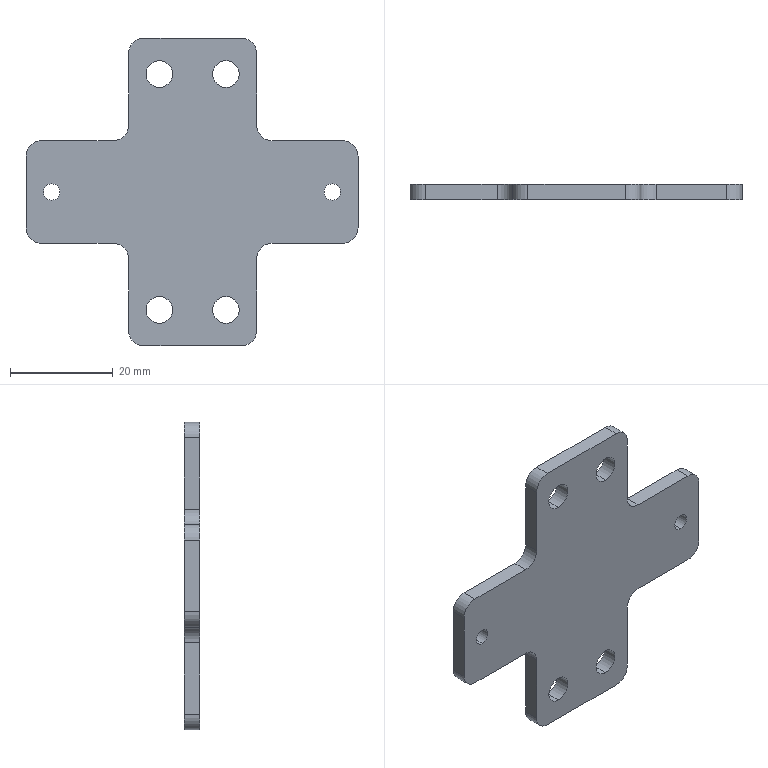Part | SolidWorks | features BaseBody 1 | 1 solid | 38 faces | box 64.75 x 3 x 60 mm | volume 6559 mm3 | cylinder 24 | plane 14 | commonest cylinder face diameters 6 x12 5.2 x8 3.2 x4
STEP:
#1=CARTESIAN_POINT('',(39.75,0.,-31.6));
#2=VERTEX_POINT('',#1);
#3=CARTESIAN_POINT('',(39.75,0.,-28.4));
#4=VERTEX_POINT('',#3);
#5=CARTESIAN_POINT('',(39.75,0.,-30.));
#6=DIRECTION('',(0.,1.,0.));
#7=DIRECTION('',(0.,0.,1.));
#8=AXIS2_PLACEMENT_3D('',#5,#6,#7);
#9=CIRCLE('',#8,1.6);
#10=EDGE_CURVE('',#2,#4,#9,.T.);
#11=ORIENTED_EDGE('',*,*,#10,.F.);
#12=CARTESIAN_POINT('',(39.75,3.,-31.6));
#13=VERTEX_POINT('',#12);
#14=CARTESIAN_POINT('',(39.75,-28.284,-31.6));
#15=DIRECTION('',(0.,1.,0.));
#16=VECTOR('',#15,1000.);
#17=LINE('',#14,#16);
#18=EDGE_CURVE('',#2,#13,#17,.T.);
#19=ORIENTED_EDGE('',*,*,#18,.T.);
#20=CARTESIAN_POINT('',(39.75,3.,-28.4));
#21=VERTEX_POINT('',#20);
#22=CARTESIAN_POINT('',(39.75,3.,-30.));
#23=DIRECTION('',(0.,-1.,0.));
#24=DIRECTION('',(0.,0.,1.));
#25=AXIS2_PLACEMENT_3D('',#22,#23,#24);
#26=CIRCLE('',#25,1.6);
#27=EDGE_CURVE('',#21,#13,#26,.T.);
#28=ORIENTED_EDGE('',*,*,#27,.F.);
#29=CARTESIAN_POINT('',(39.75,-28.284,-28.4));
#30=DIRECTION('',(0.,1.,0.));
#31=VECTOR('',#30,1000.);
#32=LINE('',#29,#31);
#33=EDGE_CURVE('',#4,#21,#32,.T.);
#34=ORIENTED_EDGE('',*,*,#33,.F.);
#35=EDGE_LOOP('',(#11,#19,#28,#34));
#36=FACE_OUTER_BOUND('',#35,.T.);
#37=CARTESIAN_POINT('',(39.75,-28.284,-30.));
#38=DIRECTION('',(0.,1.,0.));
#39=DIRECTION('',(0.,0.,1.));
#40=AXIS2_PLACEMENT_3D('',#37,#38,#39);
#41=CYLINDRICAL_SURFACE('',#40,1.6);
#42=ADVANCED_FACE('',(#36),#41,.F.);
#43=CARTESIAN_POINT('',(-15.,0.,-31.6));
#44=VERTEX_POINT('',#43);
#45=CARTESIAN_POINT('',(-15.,0.,-28.4));
#46=VERTEX_POINT('',#45);
#47=CARTESIAN_POINT('',(-15.,0.,-30.));
#48=DIRECTION('',(0.,1.,0.));
#49=DIRECTION('',(0.,0.,1.));
#50=AXIS2_PLACEMENT_3D('',#47,#48,#49);
#51=CIRCLE('',#50,1.6);
#52=EDGE_CURVE('',#44,#46,#51,.T.);
#53=ORIENTED_EDGE('',*,*,#52,.F.);
#54=CARTESIAN_POINT('',(-15.,3.,-31.6));
#55=VERTEX_POINT('',#54);
#56=CARTESIAN_POINT('',(-15.,-28.284,-31.6));
#57=DIRECTION('',(0.,1.,0.));
#58=VECTOR('',#57,1000.);
#59=LINE('',#56,#58);
#60=EDGE_CURVE('',#44,#55,#59,.T.);
#61=ORIENTED_EDGE('',*,*,#60,.T.);
#62=CARTESIAN_POINT('',(-15.,3.,-28.4));
#63=VERTEX_POINT('',#62);
#64=CARTESIAN_POINT('',(-15.,3.,-30.));
#65=DIRECTION('',(0.,-1.,0.));
#66=DIRECTION('',(0.,0.,1.));
#67=AXIS2_PLACEMENT_3D('',#64,#65,#66);
#68=CIRCLE('',#67,1.6);
#69=EDGE_CURVE('',#63,#55,#68,.T.);
#70=ORIENTED_EDGE('',*,*,#69,.F.);
#71=CARTESIAN_POINT('',(-15.,-28.284,-28.4));
#72=DIRECTION('',(0.,1.,0.));
#73=VECTOR('',#72,1000.);
#74=LINE('',#71,#73);
#75=EDGE_CURVE('',#46,#63,#74,.T.);
#76=ORIENTED_EDGE('',*,*,#75,.F.);
#77=EDGE_LOOP('',(#53,#61,#70,#76));
#78=FACE_OUTER_BOUND('',#77,.T.);
#79=CARTESIAN_POINT('',(-15.,-28.284,-30.));
#80=DIRECTION('',(0.,1.,0.));
#81=DIRECTION('',(0.,0.,1.));
#82=AXIS2_PLACEMENT_3D('',#79,#80,#81);
#83=CYLINDRICAL_SURFACE('',#82,1.6);
#84=ADVANCED_FACE('',(#78),#83,.F.);
#85=CARTESIAN_POINT('',(19.,3.,-50.4));
#86=VERTEX_POINT('',#85);
#87=CARTESIAN_POINT('',(19.,3.,-55.6));
#88=VERTEX_POINT('',#87);
#89=CARTESIAN_POINT('',(19.,3.,-53.));
#90=DIRECTION('',(0.,-1.,0.));
#91=DIRECTION('',(0.,0.,-1.));
#92=AXIS2_PLACEMENT_3D('',#89,#90,#91);
#93=CIRCLE('',#92,2.6);
#94=EDGE_CURVE('',#86,#88,#93,.T.);
#95=ORIENTED_EDGE('',*,*,#94,.F.);
#96=CARTESIAN_POINT('',(19.,0.,-50.4));
#97=VERTEX_POINT('',#96);
#98=CARTESIAN_POINT('',(19.,3.,-50.4));
#99=DIRECTION('',(0.,-1.,0.));
#100=VECTOR('',#99,1000.);
#101=LINE('',#98,#100);
#102=EDGE_CURVE('',#86,#97,#101,.T.);
#103=ORIENTED_EDGE('',*,*,#102,.T.);
#104=CARTESIAN_POINT('',(19.,0.,-55.6));
#105=VERTEX_POINT('',#104);
#106=CARTESIAN_POINT('',(19.,0.,-53.));
#107=DIRECTION('',(0.,1.,0.));
#108=DIRECTION('',(0.,0.,-1.));
#109=AXIS2_PLACEMENT_3D('',#106,#107,#108);
#110=CIRCLE('',#109,2.6);
#111=EDGE_CURVE('',#105,#97,#110,.T.);
#112=ORIENTED_EDGE('',*,*,#111,.F.);
#113=CARTESIAN_POINT('',(19.,3.,-55.6));
#114=DIRECTION('',(0.,-1.,0.));
#115=VECTOR('',#114,1000.);
#116=LINE('',#113,#115);
#117=EDGE_CURVE('',#88,#105,#116,.T.);
#118=ORIENTED_EDGE('',*,*,#117,.F.);
#119=EDGE_LOOP('',(#95,#103,#112,#118));
#120=FACE_OUTER_BOUND('',#119,.T.);
#121=CARTESIAN_POINT('',(19.,3.,-53.));
#122=DIRECTION('',(0.,-1.,0.));
#123=DIRECTION('',(0.,0.,-1.));
#124=AXIS2_PLACEMENT_3D('',#121,#122,#123);
#125=CYLINDRICAL_SURFACE('',#124,2.6);
#126=ADVANCED_FACE('',(#120),#125,.F.);
#127=CARTESIAN_POINT('',(19.,3.,-4.4));
#128=VERTEX_POINT('',#127);
#129=CARTESIAN_POINT('',(19.,3.,-9.6));
#130=VERTEX_POINT('',#129);
#131=CARTESIAN_POINT('',(19.,3.,-7.));
#132=DIRECTION('',(0.,-1.,0.));
#133=DIRECTION('',(0.,0.,-1.));
#134=AXIS2_PLACEMENT_3D('',#131,#132,#133);
#135=CIRCLE('',#134,2.6);
#136=EDGE_CURVE('',#128,#130,#135,.T.);
#137=ORIENTED_EDGE('',*,*,#136,.F.);
#138=CARTESIAN_POINT('',(19.,0.,-4.4));
#139=VERTEX_POINT('',#138);
#140=CARTESIAN_POINT('',(19.,3.,-4.4));
#141=DIRECTION('',(0.,-1.,0.));
#142=VECTOR('',#141,1000.);
#143=LINE('',#140,#142);
#144=EDGE_CURVE('',#128,#139,#143,.T.);
#145=ORIENTED_EDGE('',*,*,#144,.T.);
#146=CARTESIAN_POINT('',(19.,0.,-9.6));
#147=VERTEX_POINT('',#146);
#148=CARTESIAN_POINT('',(19.,0.,-7.));
#149=DIRECTION('',(0.,1.,0.));
#150=DIRECTION('',(0.,0.,-1.));
#151=AXIS2_PLACEMENT_3D('',#148,#149,#150);
#152=CIRCLE('',#151,2.6);
#153=EDGE_CURVE('',#147,#139,#152,.T.);
#154=ORIENTED_EDGE('',*,*,#153,.F.);
#155=CARTESIAN_POINT('',(19.,3.,-9.6));
#156=DIRECTION('',(0.,-1.,0.));
#157=VECTOR('',#156,1000.);
#158=LINE('',#155,#157);
#159=EDGE_CURVE('',#130,#147,#158,.T.);
#160=ORIENTED_EDGE('',*,*,#159,.F.);
#161=EDGE_LOOP('',(#137,#145,#154,#160));
#162=FACE_OUTER_BOUND('',#161,.T.);
#163=CARTESIAN_POINT('',(19.,3.,-7.));
#164=DIRECTION('',(0.,-1.,0.));
#165=DIRECTION('',(0.,0.,-1.));
#166=AXIS2_PLACEMENT_3D('',#163,#164,#165);
#167=CYLINDRICAL_SURFACE('',#166,2.6);
#168=ADVANCED_FACE('',(#162),#167,.F.);
#169=CARTESIAN_POINT('',(6.,3.,-4.4));
#170=VERTEX_POINT('',#169);
#171=CARTESIAN_POINT('',(6.,3.,-9.6));
#172=VERTEX_POINT('',#171);
#173=CARTESIAN_POINT('',(6.,3.,-7.));
#174=DIRECTION('',(0.,-1.,0.));
#175=DIRECTION('',(0.,0.,-1.));
#176=AXIS2_PLACEMENT_3D('',#173,#174,#175);
#177=CIRCLE('',#176,2.6);
#178=EDGE_CURVE('',#170,#172,#177,.T.);
#179=ORIENTED_EDGE('',*,*,#178,.F.);
#180=CARTESIAN_POINT('',(6.,0.,-4.4));
#181=VERTEX_POINT('',#180);
#182=CARTESIAN_POINT('',(6.,3.,-4.4));
#183=DIRECTION('',(0.,-1.,0.));
#184=VECTOR('',#183,1000.);
#185=LINE('',#182,#184);
#186=EDGE_CURVE('',#170,#181,#185,.T.);
#187=ORIENTED_EDGE('',*,*,#186,.T.);
#188=CARTESIAN_POINT('',(6.,0.,-9.6));
#189=VERTEX_POINT('',#188);
#190=CARTESIAN_POINT('',(6.,0.,-7.));
#191=DIRECTION('',(0.,1.,0.));
#192=DIRECTION('',(0.,0.,-1.));
#193=AXIS2_PLACEMENT_3D('',#190,#191,#192);
#194=CIRCLE('',#193,2.6);
#195=EDGE_CURVE('',#189,#181,#194,.T.);
#196=ORIENTED_EDGE('',*,*,#195,.F.);
#197=CARTESIAN_POINT('',(6.,3.,-9.6));
#198=DIRECTION('',(0.,-1.,0.));
#199=VECTOR('',#198,1000.);
#200=LINE('',#197,#199);
#201=EDGE_CURVE('',#172,#189,#200,.T.);
#202=ORIENTED_EDGE('',*,*,#201,.F.);
#203=EDGE_LOOP('',(#179,#187,#196,#202));
#204=FACE_OUTER_BOUND('',#203,.T.);
#205=CARTESIAN_POINT('',(6.,3.,-7.));
#206=DIRECTION('',(0.,-1.,0.));
#207=DIRECTION('',(0.,0.,-1.));
#208=AXIS2_PLACEMENT_3D('',#205,#206,#207);
#209=CYLINDRICAL_SURFACE('',#208,2.6);
#210=ADVANCED_FACE('',(#204),#209,.F.);
#211=CARTESIAN_POINT('',(6.,3.,-50.4));
#212=VERTEX_POINT('',#211);
#213=CARTESIAN_POINT('',(6.,3.,-55.6));
#214=VERTEX_POINT('',#213);
#215=CARTESIAN_POINT('',(6.,3.,-53.));
#216=DIRECTION('',(0.,-1.,0.));
#217=DIRECTION('',(0.,0.,-1.));
#218=AXIS2_PLACEMENT_3D('',#215,#216,#217);
#219=CIRCLE('',#218,2.6);
#220=EDGE_CURVE('',#212,#214,#219,.T.);
#221=ORIENTED_EDGE('',*,*,#220,.F.);
#222=CARTESIAN_POINT('',(6.,0.,-50.4));
#223=VERTEX_POINT('',#222);
#224=CARTESIAN_POINT('',(6.,3.,-50.4));
#225=DIRECTION('',(0.,-1.,0.));
#226=VECTOR('',#225,1000.);
#227=LINE('',#224,#226);
#228=EDGE_CURVE('',#212,#223,#227,.T.);
#229=ORIENTED_EDGE('',*,*,#228,.T.);
#230=CARTESIAN_POINT('',(6.,0.,-55.6));
#231=VERTEX_POINT('',#230);
#232=CARTESIAN_POINT('',(6.,0.,-53.));
#233=DIRECTION('',(0.,1.,0.));
#234=DIRECTION('',(0.,0.,-1.));
#235=AXIS2_PLACEMENT_3D('',#232,#233,#234);
#236=CIRCLE('',#235,2.6);
#237=EDGE_CURVE('',#231,#223,#236,.T.);
#238=ORIENTED_EDGE('',*,*,#237,.F.);
#239=CARTESIAN_POINT('',(6.,3.,-55.6));
#240=DIRECTION('',(0.,-1.,0.));
#241=VECTOR('',#240,1000.);
#242=LINE('',#239,#241);
#243=EDGE_CURVE('',#214,#231,#242,.T.);
#244=ORIENTED_EDGE('',*,*,#243,.F.);
#245=EDGE_LOOP('',(#221,#229,#238,#244));
#246=FACE_OUTER_BOUND('',#245,.T.);
#247=CARTESIAN_POINT('',(6.,3.,-53.));
#248=DIRECTION('',(0.,-1.,0.));
#249=DIRECTION('',(0.,0.,-1.));
#250=AXIS2_PLACEMENT_3D('',#247,#248,#249);
#251=CYLINDRICAL_SURFACE('',#250,2.6);
#252=ADVANCED_FACE('',(#246),#251,.F.);
#253=CARTESIAN_POINT('',(39.75,0.,-30.));
#254=DIRECTION('',(0.,1.,0.));
#255=DIRECTION('',(0.,0.,1.));
#256=AXIS2_PLACEMENT_3D('',#253,#254,#255);
#257=CIRCLE('',#256,1.6);
#258=EDGE_CURVE('',#4,#2,#257,.T.);
#259=ORIENTED_EDGE('',*,*,#258,.T.);
#260=ORIENTED_EDGE('',*,*,#10,.T.);
#261=EDGE_LOOP('',(#259,#260));
#262=FACE_BOUND('',#261,.T.);
#263=CARTESIAN_POINT('',(-15.,0.,-30.));
#264=DIRECTION('',(0.,1.,0.));
#265=DIRECTION('',(0.,0.,1.));
#266=AXIS2_PLACEMENT_3D('',#263,#264,#265);
#267=CIRCLE('',#266,1.6);
#268=EDGE_CURVE('',#46,#44,#267,.T.);
#269=ORIENTED_EDGE('',*,*,#268,.T.);
#270=ORIENTED_EDGE('',*,*,#52,.T.);
#271=EDGE_LOOP('',(#269,#270));
#272=FACE_BOUND('',#271,.T.);
#273=ORIENTED_EDGE('',*,*,#111,.T.);
#274=CARTESIAN_POINT('',(19.,0.,-53.));
#275=DIRECTION('',(0.,1.,0.));
#276=DIRECTION('',(0.,0.,-1.));
#277=AXIS2_PLACEMENT_3D('',#274,#275,#276);
#278=CIRCLE('',#277,2.6);
#279=EDGE_CURVE('',#97,#105,#278,.T.);
#280=ORIENTED_EDGE('',*,*,#279,.T.);
#281=EDGE_LOOP('',(#273,#280));
#282=FACE_BOUND('',#281,.T.);
#283=ORIENTED_EDGE('',*,*,#153,.T.);
#284=CARTESIAN_POINT('',(19.,0.,-7.));
#285=DIRECTION('',(0.,1.,0.));
#286=DIRECTION('',(0.,0.,-1.));
#287=AXIS2_PLACEMENT_3D('',#284,#285,#286);
#288=CIRCLE('',#287,2.6);
#289=EDGE_CURVE('',#139,#147,#288,.T.);
#290=ORIENTED_EDGE('',*,*,#289,.T.);
#291=EDGE_LOOP('',(#283,#290));
#292=FACE_BOUND('',#291,.T.);
#293=CARTESIAN_POINT('',(28.,0.,-40.));
#294=VERTEX_POINT('',#293);
#295=CARTESIAN_POINT('',(41.75,0.,-40.));
#296=VERTEX_POINT('',#295);
#297=CARTESIAN_POINT('',(0.,0.,-40.));
#298=DIRECTION('',(1.,0.,0.));
#299=VECTOR('',#298,1000.);
#300=LINE('',#297,#299);
#301=EDGE_CURVE('',#294,#296,#300,.T.);
#302=ORIENTED_EDGE('',*,*,#301,.T.);
#303=CARTESIAN_POINT('',(44.75,0.,-37.));
#304=VERTEX_POINT('',#303);
#305=CARTESIAN_POINT('',(41.75,0.,-37.));
#306=DIRECTION('',(0.,-1.,0.));
#307=DIRECTION('',(0.,0.,1.));
#308=AXIS2_PLACEMENT_3D('',#305,#306,#307);
#309=CIRCLE('',#308,3.);
#310=EDGE_CURVE('',#296,#304,#309,.T.);
#311=ORIENTED_EDGE('',*,*,#310,.T.);
#312=CARTESIAN_POINT('',(44.75,0.,-23.));
#313=VERTEX_POINT('',#312);
#314=CARTESIAN_POINT('',(44.75,0.,0.));
#315=DIRECTION('',(0.,0.,1.));
#316=VECTOR('',#315,1000.);
#317=LINE('',#314,#316);
#318=EDGE_CURVE('',#304,#313,#317,.T.);
#319=ORIENTED_EDGE('',*,*,#318,.T.);
#320=CARTESIAN_POINT('',(41.75,0.,-20.));
#321=VERTEX_POINT('',#320);
#322=CARTESIAN_POINT('',(41.75,0.,-23.));
#323=DIRECTION('',(0.,-1.,0.));
#324=DIRECTION('',(0.,0.,1.));
#325=AXIS2_PLACEMENT_3D('',#322,#323,#324);
#326=CIRCLE('',#325,3.);
#327=EDGE_CURVE('',#313,#321,#326,.T.);
#328=ORIENTED_EDGE('',*,*,#327,.T.);
#329=CARTESIAN_POINT('',(28.,0.,-20.));
#330=VERTEX_POINT('',#329);
#331=CARTESIAN_POINT('',(0.,0.,-20.));
#332=DIRECTION('',(-1.,0.,0.));
#333=VECTOR('',#332,1000.);
#334=LINE('',#331,#333);
#335=EDGE_CURVE('',#321,#330,#334,.T.);
#336=ORIENTED_EDGE('',*,*,#335,.T.);
#337=CARTESIAN_POINT('',(25.,0.,-17.));
#338=VERTEX_POINT('',#337);
#339=CARTESIAN_POINT('',(28.,0.,-17.));
#340=DIRECTION('',(0.,1.,0.));
#341=DIRECTION('',(0.,0.,1.));
#342=AXIS2_PLACEMENT_3D('',#339,#340,#341);
#343=CIRCLE('',#342,3.);
#344=EDGE_CURVE('',#330,#338,#343,.T.);
#345=ORIENTED_EDGE('',*,*,#344,.T.);
#346=CARTESIAN_POINT('',(25.,0.,-3.));
#347=VERTEX_POINT('',#346);
#348=CARTESIAN_POINT('',(25.,0.,0.));
#349=DIRECTION('',(0.,0.,1.));
#350=VECTOR('',#349,1000.);
#351=LINE('',#348,#350);
#352=EDGE_CURVE('',#338,#347,#351,.T.);
#353=ORIENTED_EDGE('',*,*,#352,.T.);
#354=CARTESIAN_POINT('',(22.,0.,0.));
#355=VERTEX_POINT('',#354);
#356=CARTESIAN_POINT('',(22.,0.,-3.));
#357=DIRECTION('',(0.,-1.,0.));
#358=DIRECTION('',(0.,0.,-1.));
#359=AXIS2_PLACEMENT_3D('',#356,#357,#358);
#360=CIRCLE('',#359,3.);
#361=EDGE_CURVE('',#347,#355,#360,.T.);
#362=ORIENTED_EDGE('',*,*,#361,.T.);
#363=CARTESIAN_POINT('',(3.,0.,0.));
#364=VERTEX_POINT('',#363);
#365=CARTESIAN_POINT('',(0.,0.,0.));
#366=DIRECTION('',(-1.,0.,0.));
#367=VECTOR('',#366,1000.);
#368=LINE('',#365,#367);
#369=EDGE_CURVE('',#355,#364,#368,.T.);
#370=ORIENTED_EDGE('',*,*,#369,.T.);
#371=CARTESIAN_POINT('',(0.,0.,-3.));
#372=VERTEX_POINT('',#371);
#373=CARTESIAN_POINT('',(3.,0.,-3.));
#374=DIRECTION('',(0.,-1.,0.));
#375=DIRECTION('',(0.,0.,-1.));
#376=AXIS2_PLACEMENT_3D('',#373,#374,#375);
#377=CIRCLE('',#376,3.);
#378=EDGE_CURVE('',#364,#372,#377,.T.);
#379=ORIENTED_EDGE('',*,*,#378,.T.);
#380=CARTESIAN_POINT('',(0.,0.,-17.));
#381=VERTEX_POINT('',#380);
#382=CARTESIAN_POINT('',(0.,0.,0.));
#383=DIRECTION('',(0.,0.,-1.));
#384=VECTOR('',#383,1000.);
#385=LINE('',#382,#384);
#386=EDGE_CURVE('',#372,#381,#385,.T.);
#387=ORIENTED_EDGE('',*,*,#386,.T.);
#388=CARTESIAN_POINT('',(-3.,0.,-20.));
#389=VERTEX_POINT('',#388);
#390=CARTESIAN_POINT('',(-3.,0.,-17.));
#391=DIRECTION('',(0.,1.,0.));
#392=DIRECTION('',(0.,0.,1.));
#393=AXIS2_PLACEMENT_3D('',#390,#391,#392);
#394=CIRCLE('',#393,3.);
#395=EDGE_CURVE('',#381,#389,#394,.T.);
#396=ORIENTED_EDGE('',*,*,#395,.T.);
#397=CARTESIAN_POINT('',(-17.,0.,-20.));
#398=VERTEX_POINT('',#397);
#399=CARTESIAN_POINT('',(0.,0.,-20.));
#400=DIRECTION('',(-1.,0.,0.));
#401=VECTOR('',#400,1000.);
#402=LINE('',#399,#401);
#403=EDGE_CURVE('',#389,#398,#402,.T.);
#404=ORIENTED_EDGE('',*,*,#403,.T.);
#405=CARTESIAN_POINT('',(-20.,0.,-23.));
#406=VERTEX_POINT('',#405);
#407=CARTESIAN_POINT('',(-17.,0.,-23.));
#408=DIRECTION('',(0.,-1.,0.));
#409=DIRECTION('',(0.,0.,1.));
#410=AXIS2_PLACEMENT_3D('',#407,#408,#409);
#411=CIRCLE('',#410,3.);
#412=EDGE_CURVE('',#398,#406,#411,.T.);
#413=ORIENTED_EDGE('',*,*,#412,.T.);
#414=CARTESIAN_POINT('',(-20.,0.,-37.));
#415=VERTEX_POINT('',#414);
#416=CARTESIAN_POINT('',(-20.,0.,0.));
#417=DIRECTION('',(0.,0.,-1.));
#418=VECTOR('',#417,1000.);
#419=LINE('',#416,#418);
#420=EDGE_CURVE('',#406,#415,#419,.T.);
#421=ORIENTED_EDGE('',*,*,#420,.T.);
#422=CARTESIAN_POINT('',(-17.,0.,-40.));
#423=VERTEX_POINT('',#422);
#424=CARTESIAN_POINT('',(-17.,0.,-37.));
#425=DIRECTION('',(0.,-1.,0.));
#426=DIRECTION('',(0.,0.,1.));
#427=AXIS2_PLACEMENT_3D('',#424,#425,#426);
#428=CIRCLE('',#427,3.);
#429=EDGE_CURVE('',#415,#423,#428,.T.);
#430=ORIENTED_EDGE('',*,*,#429,.T.);
#431=CARTESIAN_POINT('',(-3.,0.,-40.));
#432=VERTEX_POINT('',#431);
#433=CARTESIAN_POINT('',(0.,0.,-40.));
#434=DIRECTION('',(1.,0.,0.));
#435=VECTOR('',#434,1000.);
#436=LINE('',#433,#435);
#437=EDGE_CURVE('',#423,#432,#436,.T.);
#438=ORIENTED_EDGE('',*,*,#437,.T.);
#439=CARTESIAN_POINT('',(0.,0.,-43.));
#440=VERTEX_POINT('',#439);
#441=CARTESIAN_POINT('',(-3.,0.,-43.));
#442=DIRECTION('',(0.,1.,0.));
#443=DIRECTION('',(0.,0.,1.));
#444=AXIS2_PLACEMENT_3D('',#441,#442,#443);
#445=CIRCLE('',#444,3.);
#446=EDGE_CURVE('',#432,#440,#445,.T.);
#447=ORIENTED_EDGE('',*,*,#446,.T.);
#448=CARTESIAN_POINT('',(0.,0.,-57.));
#449=VERTEX_POINT('',#448);
#450=CARTESIAN_POINT('',(0.,0.,0.));
#451=DIRECTION('',(0.,0.,-1.));
#452=VECTOR('',#451,1000.);
#453=LINE('',#450,#452);
#454=EDGE_CURVE('',#440,#449,#453,.T.);
#455=ORIENTED_EDGE('',*,*,#454,.T.);
#456=CARTESIAN_POINT('',(3.,0.,-60.));
#457=VERTEX_POINT('',#456);
#458=CARTESIAN_POINT('',(3.,0.,-57.));
#459=DIRECTION('',(0.,-1.,0.));
#460=DIRECTION('',(0.,0.,-1.));
#461=AXIS2_PLACEMENT_3D('',#458,#459,#460);
#462=CIRCLE('',#461,3.);
#463=EDGE_CURVE('',#449,#457,#462,.T.);
#464=ORIENTED_EDGE('',*,*,#463,.T.);
#465=CARTESIAN_POINT('',(22.,0.,-60.));
#466=VERTEX_POINT('',#465);
#467=CARTESIAN_POINT('',(0.,0.,-60.));
#468=DIRECTION('',(1.,0.,0.));
#469=VECTOR('',#468,1000.);
#470=LINE('',#467,#469);
#471=EDGE_CURVE('',#457,#466,#470,.T.);
#472=ORIENTED_EDGE('',*,*,#471,.T.);
#473=CARTESIAN_POINT('',(25.,0.,-57.));
#474=VERTEX_POINT('',#473);
#475=CARTESIAN_POINT('',(22.,0.,-57.));
#476=DIRECTION('',(0.,-1.,0.));
#477=DIRECTION('',(0.,0.,-1.));
#478=AXIS2_PLACEMENT_3D('',#475,#476,#477);
#479=CIRCLE('',#478,3.);
#480=EDGE_CURVE('',#466,#474,#479,.T.);
#481=ORIENTED_EDGE('',*,*,#480,.T.);
#482=CARTESIAN_POINT('',(25.,0.,-43.));
#483=VERTEX_POINT('',#482);
#484=CARTESIAN_POINT('',(25.,0.,0.));
#485=DIRECTION('',(0.,0.,1.));
#486=VECTOR('',#485,1000.);
#487=LINE('',#484,#486);
#488=EDGE_CURVE('',#474,#483,#487,.T.);
#489=ORIENTED_EDGE('',*,*,#488,.T.);
#490=CARTESIAN_POINT('',(28.,0.,-43.));
#491=DIRECTION('',(0.,1.,0.));
#492=DIRECTION('',(0.,0.,1.));
#493=AXIS2_PLACEMENT_3D('',#490,#491,#492);
#494=CIRCLE('',#493,3.);
#495=EDGE_CURVE('',#483,#294,#494,.T.);
#496=ORIENTED_EDGE('',*,*,#495,.T.);
#497=EDGE_LOOP('',(#302,#311,#319,#328,#336,#345,#353,#362,#370,#379,#387,#396,#404,#413,#421,#430,#438,#447,#455,#464,#472,#481,#489,#496));
#498=FACE_OUTER_BOUND('',#497,.T.);
#499=ORIENTED_EDGE('',*,*,#195,.T.);
#500=CARTESIAN_POINT('',(6.,0.,-7.));
#501=DIRECTION('',(0.,1.,0.));
#502=DIRECTION('',(0.,0.,-1.));
#503=AXIS2_PLACEMENT_3D('',#500,#501,#502);
#504=CIRCLE('',#503,2.6);
#505=EDGE_CURVE('',#181,#189,#504,.T.);
#506=ORIENTED_EDGE('',*,*,#505,.T.);
#507=EDGE_LOOP('',(#499,#506));
#508=FACE_BOUND('',#507,.T.);
#509=ORIENTED_EDGE('',*,*,#237,.T.);
#510=CARTESIAN_POINT('',(6.,0.,-53.));
#511=DIRECTION('',(0.,1.,0.));
#512=DIRECTION('',(0.,0.,-1.));
#513=AXIS2_PLACEMENT_3D('',#510,#511,#512);
#514=CIRCLE('',#513,2.6);
#515=EDGE_CURVE('',#223,#231,#514,.T.);
#516=ORIENTED_EDGE('',*,*,#515,.T.);
#517=EDGE_LOOP('',(#509,#516));
#518=FACE_BOUND('',#517,.T.);
#519=CARTESIAN_POINT('',(0.,0.,0.));
#520=DIRECTION('',(0.,-1.,0.));
#521=DIRECTION('',(0.,0.,-1.));
#522=AXIS2_PLACEMENT_3D('',#519,#520,#521);
#523=PLANE('',#522);
#524=ADVANCED_FACE('',(#262,#272,#282,#292,#498,#508,#518),#523,.T.);
#525=ORIENTED_EDGE('',*,*,#18,.F.);
#526=ORIENTED_EDGE('',*,*,#258,.F.);
#527=ORIENTED_EDGE('',*,*,#33,.T.);
#528=CARTESIAN_POINT('',(39.75,3.,-30.));
#529=DIRECTION('',(0.,-1.,0.));
#530=DIRECTION('',(0.,0.,1.));
#531=AXIS2_PLACEMENT_3D('',#528,#529,#530);
#532=CIRCLE('',#531,1.6);
#533=EDGE_CURVE('',#13,#21,#532,.T.);
#534=ORIENTED_EDGE('',*,*,#533,.F.);
#535=EDGE_LOOP('',(#525,#526,#527,#534));
#536=FACE_OUTER_BOUND('',#535,.T.);
#537=CARTESIAN_POINT('',(39.75,-28.284,-30.));
#538=DIRECTION('',(0.,1.,0.));
#539=DIRECTION('',(0.,0.,1.));
#540=AXIS2_PLACEMENT_3D('',#537,#538,#539);
#541=CYLINDRICAL_SURFACE('',#540,1.6);
#542=ADVANCED_FACE('',(#536),#541,.F.);
#543=ORIENTED_EDGE('',*,*,#60,.F.);
#544=ORIENTED_EDGE('',*,*,#268,.F.);
#545=ORIENTED_EDGE('',*,*,#75,.T.);
#546=CARTESIAN_POINT('',(-15.,3.,-30.));
#547=DIRECTION('',(0.,-1.,0.));
#548=DIRECTION('',(0.,0.,1.));
#549=AXIS2_PLACEMENT_3D('',#546,#547,#548);
#550=CIRCLE('',#549,1.6);
#551=EDGE_CURVE('',#55,#63,#550,.T.);
#552=ORIENTED_EDGE('',*,*,#551,.F.);
#553=EDGE_LOOP('',(#543,#544,#545,#552));
#554=FACE_OUTER_BOUND('',#553,.T.);
#555=CARTESIAN_POINT('',(-15.,-28.284,-30.));
#556=DIRECTION('',(0.,1.,0.));
#557=DIRECTION('',(0.,0.,1.));
#558=AXIS2_PLACEMENT_3D('',#555,#556,#557);
#559=CYLINDRICAL_SURFACE('',#558,1.6);
#560=ADVANCED_FACE('',(#554),#559,.F.);
#561=ORIENTED_EDGE('',*,*,#102,.F.);
#562=CARTESIAN_POINT('',(19.,3.,-53.));
#563=DIRECTION('',(0.,-1.,0.));
#564=DIRECTION('',(0.,0.,-1.));
#565=AXIS2_PLACEMENT_3D('',#562,#563,#564);
#566=CIRCLE('',#565,2.6);
#567=EDGE_CURVE('',#88,#86,#566,.T.);
#568=ORIENTED_EDGE('',*,*,#567,.F.);
#569=ORIENTED_EDGE('',*,*,#117,.T.);
#570=ORIENTED_EDGE('',*,*,#279,.F.);
#571=EDGE_LOOP('',(#561,#568,#569,#570));
#572=FACE_OUTER_BOUND('',#571,.T.);
#573=CARTESIAN_POINT('',(19.,3.,-53.));
#574=DIRECTION('',(0.,-1.,0.));
#575=DIRECTION('',(0.,0.,-1.));
#576=AXIS2_PLACEMENT_3D('',#573,#574,#575);
#577=CYLINDRICAL_SURFACE('',#576,2.6);
#578=ADVANCED_FACE('',(#572),#577,.F.);
#579=ORIENTED_EDGE('',*,*,#144,.F.);
#580=CARTESIAN_POINT('',(19.,3.,-7.));
#581=DIRECTION('',(0.,-1.,0.));
#582=DIRECTION('',(0.,0.,-1.));
#583=AXIS2_PLACEMENT_3D('',#580,#581,#582);
#584=CIRCLE('',#583,2.6);
#585=EDGE_CURVE('',#130,#128,#584,.T.);
#586=ORIENTED_EDGE('',*,*,#585,.F.);
#587=ORIENTED_EDGE('',*,*,#159,.T.);
#588=ORIENTED_EDGE('',*,*,#289,.F.);
#589=EDGE_LOOP('',(#579,#586,#587,#588));
#590=FACE_OUTER_BOUND('',#589,.T.);
#591=CARTESIAN_POINT('',(19.,3.,-7.));
#592=DIRECTION('',(0.,-1.,0.));
#593=DIRECTION('',(0.,0.,-1.));
#594=AXIS2_PLACEMENT_3D('',#591,#592,#593);
#595=CYLINDRICAL_SURFACE('',#594,2.6);
#596=ADVANCED_FACE('',(#590),#595,.F.);
#597=CARTESIAN_POINT('',(41.75,3.,-40.));
#598=VERTEX_POINT('',#597);
#599=CARTESIAN_POINT('',(44.75,3.,-37.));
#600=VERTEX_POINT('',#599);
#601=CARTESIAN_POINT('',(41.75,3.,-37.));
#602=DIRECTION('',(0.,-1.,0.));
#603=DIRECTION('',(0.,0.,1.));
#604=AXIS2_PLACEMENT_3D('',#601,#602,#603);
#605=CIRCLE('',#604,3.);
#606=EDGE_CURVE('',#598,#600,#605,.T.);
#607=ORIENTED_EDGE('',*,*,#606,.T.);
#608=CARTESIAN_POINT('',(44.75,-28.284,-37.));
#609=DIRECTION('',(0.,-1.,0.));
#610=VECTOR('',#609,1000.);
#611=LINE('',#608,#610);
#612=EDGE_CURVE('',#600,#304,#611,.T.);
#613=ORIENTED_EDGE('',*,*,#612,.T.);
#614=ORIENTED_EDGE('',*,*,#310,.F.);
#615=CARTESIAN_POINT('',(41.75,-28.284,-40.));
#616=DIRECTION('',(0.,1.,0.));
#617=VECTOR('',#616,1000.);
#618=LINE('',#615,#617);
#619=EDGE_CURVE('',#296,#598,#618,.T.);
#620=ORIENTED_EDGE('',*,*,#619,.T.);
#621=EDGE_LOOP('',(#607,#613,#614,#620));
#622=FACE_OUTER_BOUND('',#621,.T.);
#623=CARTESIAN_POINT('',(41.75,-28.284,-37.));
#624=DIRECTION('',(0.,1.,0.));
#625=DIRECTION('',(0.,0.,1.));
#626=AXIS2_PLACEMENT_3D('',#623,#624,#625);
#627=CYLINDRICAL_SURFACE('',#626,3.);
#628=ADVANCED_FACE('',(#622),#627,.T.);
#629=ORIENTED_EDGE('',*,*,#301,.F.);
#630=CARTESIAN_POINT('',(28.,3.,-40.));
#631=VERTEX_POINT('',#630);
#632=CARTESIAN_POINT('',(28.,-28.284,-40.));
#633=DIRECTION('',(0.,1.,0.));
#634=VECTOR('',#633,1000.);
#635=LINE('',#632,#634);
#636=EDGE_CURVE('',#294,#631,#635,.T.);
#637=ORIENTED_EDGE('',*,*,#636,.T.);
#638=CARTESIAN_POINT('',(25.,3.,-40.));
#639=DIRECTION('',(1.,0.,0.));
#640=VECTOR('',#639,1000.);
#641=LINE('',#638,#640);
#642=EDGE_CURVE('',#631,#598,#641,.T.);
#643=ORIENTED_EDGE('',*,*,#642,.T.);
#644=ORIENTED_EDGE('',*,*,#619,.F.);
#645=EDGE_LOOP('',(#629,#637,#643,#644));
#646=FACE_OUTER_BOUND('',#645,.T.);
#647=CARTESIAN_POINT('',(25.,-28.284,-40.));
#648=DIRECTION('',(0.,0.,-1.));
#649=DIRECTION('',(-1.,0.,0.));
#650=AXIS2_PLACEMENT_3D('',#647,#648,#649);
#651=PLANE('',#650);
#652=ADVANCED_FACE('',(#646),#651,.T.);
#653=CARTESIAN_POINT('',(25.,3.,-43.));
#654=VERTEX_POINT('',#653);
#655=CARTESIAN_POINT('',(25.,-28.284,-43.));
#656=DIRECTION('',(0.,-1.,0.));
#657=VECTOR('',#656,1000.);
#658=LINE('',#655,#657);
#659=EDGE_CURVE('',#654,#483,#658,.T.);
#660=ORIENTED_EDGE('',*,*,#659,.F.);
#661=CARTESIAN_POINT('',(28.,3.,-43.));
#662=DIRECTION('',(0.,-1.,0.));
#663=DIRECTION('',(0.,0.,1.));
#664=AXIS2_PLACEMENT_3D('',#661,#662,#663);
#665=CIRCLE('',#664,3.);
#666=EDGE_CURVE('',#631,#654,#665,.T.);
#667=ORIENTED_EDGE('',*,*,#666,.F.);
#668=ORIENTED_EDGE('',*,*,#636,.F.);
#669=ORIENTED_EDGE('',*,*,#495,.F.);
#670=EDGE_LOOP('',(#660,#667,#668,#669));
#671=FACE_OUTER_BOUND('',#670,.T.);
#672=CARTESIAN_POINT('',(28.,-28.284,-43.));
#673=DIRECTION('',(0.,1.,0.));
#674=DIRECTION('',(0.,0.,1.));
#675=AXIS2_PLACEMENT_3D('',#672,#673,#674);
#676=CYLINDRICAL_SURFACE('',#675,3.);
#677=ADVANCED_FACE('',(#671),#676,.F.);
#678=ORIENTED_EDGE('',*,*,#659,.T.);
#679=ORIENTED_EDGE('',*,*,#488,.F.);
#680=CARTESIAN_POINT('',(25.,3.,-57.));
#681=VERTEX_POINT('',#680);
#682=CARTESIAN_POINT('',(25.,3.,-57.));
#683=DIRECTION('',(0.,-1.,0.));
#684=VECTOR('',#683,1000.);
#685=LINE('',#682,#684);
#686=EDGE_CURVE('',#681,#474,#685,.T.);
#687=ORIENTED_EDGE('',*,*,#686,.F.);
#688=CARTESIAN_POINT('',(25.,3.,0.));
#689=DIRECTION('',(0.,0.,-1.));
#690=VECTOR('',#689,1000.);
#691=LINE('',#688,#690);
#692=EDGE_CURVE('',#654,#681,#691,.T.);
#693=ORIENTED_EDGE('',*,*,#692,.F.);
#694=EDGE_LOOP('',(#678,#679,#687,#693));
#695=FACE_OUTER_BOUND('',#694,.T.);
#696=CARTESIAN_POINT('',(25.,3.,0.));
#697=DIRECTION('',(-1.,0.,0.));
#698=DIRECTION('',(0.,0.,1.));
#699=AXIS2_PLACEMENT_3D('',#696,#697,#698);
#700=PLANE('',#699);
#701=ADVANCED_FACE('',(#695),#700,.F.);
#702=ORIENTED_EDGE('',*,*,#480,.F.);
#703=CARTESIAN_POINT('',(22.,3.,-60.));
#704=VERTEX_POINT('',#703);
#705=CARTESIAN_POINT('',(22.,3.,-60.));
#706=DIRECTION('',(0.,1.,0.));
#707=VECTOR('',#706,1000.);
#708=LINE('',#705,#707);
#709=EDGE_CURVE('',#466,#704,#708,.T.);
#710=ORIENTED_EDGE('',*,*,#709,.T.);
#711=CARTESIAN_POINT('',(22.,3.,-57.));
#712=DIRECTION('',(0.,-1.,0.));
#713=DIRECTION('',(0.,0.,-1.));
#714=AXIS2_PLACEMENT_3D('',#711,#712,#713);
#715=CIRCLE('',#714,3.);
#716=EDGE_CURVE('',#704,#681,#715,.T.);
#717=ORIENTED_EDGE('',*,*,#716,.T.);
#718=ORIENTED_EDGE('',*,*,#686,.T.);
#719=EDGE_LOOP('',(#702,#710,#717,#718));
#720=FACE_OUTER_BOUND('',#719,.T.);
#721=CARTESIAN_POINT('',(22.,3.,-57.));
#722=DIRECTION('',(0.,-1.,0.));
#723=DIRECTION('',(0.,0.,-1.));
#724=AXIS2_PLACEMENT_3D('',#721,#722,#723);
#725=CYLINDRICAL_SURFACE('',#724,3.);
#726=ADVANCED_FACE('',(#720),#725,.T.);
#727=ORIENTED_EDGE('',*,*,#709,.F.);
#728=ORIENTED_EDGE('',*,*,#471,.F.);
#729=CARTESIAN_POINT('',(3.,3.,-60.));
#730=VERTEX_POINT('',#729);
#731=CARTESIAN_POINT('',(3.,3.,-60.));
#732=DIRECTION('',(0.,-1.,0.));
#733=VECTOR('',#732,1000.);
#734=LINE('',#731,#733);
#735=EDGE_CURVE('',#730,#457,#734,.T.);
#736=ORIENTED_EDGE('',*,*,#735,.F.);
#737=CARTESIAN_POINT('',(0.,3.,-60.));
#738=DIRECTION('',(-1.,0.,0.));
#739=VECTOR('',#738,1000.);
#740=LINE('',#737,#739);
#741=EDGE_CURVE('',#704,#730,#740,.T.);
#742=ORIENTED_EDGE('',*,*,#741,.F.);
#743=EDGE_LOOP('',(#727,#728,#736,#742));
#744=FACE_OUTER_BOUND('',#743,.T.);
#745=CARTESIAN_POINT('',(0.,3.,-60.));
#746=DIRECTION('',(0.,0.,1.));
#747=DIRECTION('',(1.,0.,0.));
#748=AXIS2_PLACEMENT_3D('',#745,#746,#747);
#749=PLANE('',#748);
#750=ADVANCED_FACE('',(#744),#749,.F.);
#751=ORIENTED_EDGE('',*,*,#463,.F.);
#752=CARTESIAN_POINT('',(0.,3.,-57.));
#753=VERTEX_POINT('',#752);
#754=CARTESIAN_POINT('',(0.,3.,-57.));
#755=DIRECTION('',(0.,1.,0.));
#756=VECTOR('',#755,1000.);
#757=LINE('',#754,#756);
#758=EDGE_CURVE('',#449,#753,#757,.T.);
#759=ORIENTED_EDGE('',*,*,#758,.T.);
#760=CARTESIAN_POINT('',(3.,3.,-57.));
#761=DIRECTION('',(0.,-1.,0.));
#762=DIRECTION('',(0.,0.,-1.));
#763=AXIS2_PLACEMENT_3D('',#760,#761,#762);
#764=CIRCLE('',#763,3.);
#765=EDGE_CURVE('',#753,#730,#764,.T.);
#766=ORIENTED_EDGE('',*,*,#765,.T.);
#767=ORIENTED_EDGE('',*,*,#735,.T.);
#768=EDGE_LOOP('',(#751,#759,#766,#767));
#769=FACE_OUTER_BOUND('',#768,.T.);
#770=CARTESIAN_POINT('',(3.,3.,-57.));
#771=DIRECTION('',(0.,-1.,0.));
#772=DIRECTION('',(0.,0.,-1.));
#773=AXIS2_PLACEMENT_3D('',#770,#771,#772);
#774=CYLINDRICAL_SURFACE('',#773,3.);
#775=ADVANCED_FACE('',(#769),#774,.T.);
#776=ORIENTED_EDGE('',*,*,#758,.F.);
#777=ORIENTED_EDGE('',*,*,#454,.F.);
#778=CARTESIAN_POINT('',(0.,3.,-43.));
#779=VERTEX_POINT('',#778);
#780=CARTESIAN_POINT('',(0.,3.,-43.));
#781=DIRECTION('',(0.,-1.,0.));
#782=VECTOR('',#781,1000.);
#783=LINE('',#780,#782);
#784=EDGE_CURVE('',#779,#440,#783,.T.);
#785=ORIENTED_EDGE('',*,*,#784,.F.);
#786=CARTESIAN_POINT('',(0.,3.,0.));
#787=DIRECTION('',(0.,0.,1.));
#788=VECTOR('',#787,1000.);
#789=LINE('',#786,#788);
#790=EDGE_CURVE('',#753,#779,#789,.T.);
#791=ORIENTED_EDGE('',*,*,#790,.F.);
#792=EDGE_LOOP('',(#776,#777,#785,#791));
#793=FACE_OUTER_BOUND('',#792,.T.);
#794=CARTESIAN_POINT('',(0.,3.,0.));
#795=DIRECTION('',(1.,0.,0.));
#796=DIRECTION('',(0.,0.,-1.));
#797=AXIS2_PLACEMENT_3D('',#794,#795,#796);
#798=PLANE('',#797);
#799=ADVANCED_FACE('',(#793),#798,.F.);
#800=CARTESIAN_POINT('',(-3.,3.,-40.));
#801=VERTEX_POINT('',#800);
#802=CARTESIAN_POINT('',(-3.,3.,-40.));
#803=DIRECTION('',(0.,-1.,0.));
#804=VECTOR('',#803,1000.);
#805=LINE('',#802,#804);
#806=EDGE_CURVE('',#801,#432,#805,.T.);
#807=ORIENTED_EDGE('',*,*,#806,.F.);
#808=CARTESIAN_POINT('',(-3.,3.,-43.));
#809=DIRECTION('',(0.,-1.,0.));
#810=DIRECTION('',(0.,0.,1.));
#811=AXIS2_PLACEMENT_3D('',#808,#809,#810);
#812=CIRCLE('',#811,3.);
#813=EDGE_CURVE('',#779,#801,#812,.T.);
#814=ORIENTED_EDGE('',*,*,#813,.F.);
#815=ORIENTED_EDGE('',*,*,#784,.T.);
#816=ORIENTED_EDGE('',*,*,#446,.F.);
#817=EDGE_LOOP('',(#807,#814,#815,#816));
#818=FACE_OUTER_BOUND('',#817,.T.);
#819=CARTESIAN_POINT('',(-3.,3.,-43.));
#820=DIRECTION('',(0.,1.,0.));
#821=DIRECTION('',(0.,0.,1.));
#822=AXIS2_PLACEMENT_3D('',#819,#820,#821);
#823=CYLINDRICAL_SURFACE('',#822,3.);
#824=ADVANCED_FACE('',(#818),#823,.F.);
#825=ORIENTED_EDGE('',*,*,#437,.F.);
#826=CARTESIAN_POINT('',(-17.,3.,-40.));
#827=VERTEX_POINT('',#826);
#828=CARTESIAN_POINT('',(-17.,-28.284,-40.));
#829=DIRECTION('',(0.,1.,0.));
#830=VECTOR('',#829,1000.);
#831=LINE('',#828,#830);
#832=EDGE_CURVE('',#423,#827,#831,.T.);
#833=ORIENTED_EDGE('',*,*,#832,.T.);
#834=CARTESIAN_POINT('',(0.,3.,-40.));
#835=DIRECTION('',(1.,0.,0.));
#836=VECTOR('',#835,1000.);
#837=LINE('',#834,#836);
#838=EDGE_CURVE('',#827,#801,#837,.T.);
#839=ORIENTED_EDGE('',*,*,#838,.T.);
#840=ORIENTED_EDGE('',*,*,#806,.T.);
#841=EDGE_LOOP('',(#825,#833,#839,#840));
#842=FACE_OUTER_BOUND('',#841,.T.);
#843=CARTESIAN_POINT('',(0.,-28.284,-40.));
#844=DIRECTION('',(0.,0.,-1.));
#845=DIRECTION('',(-1.,0.,0.));
#846=AXIS2_PLACEMENT_3D('',#843,#844,#845);
#847=PLANE('',#846);
#848=ADVANCED_FACE('',(#842),#847,.T.);
#849=CARTESIAN_POINT('',(-20.,3.,-37.));
#850=VERTEX_POINT('',#849);
#851=CARTESIAN_POINT('',(-17.,3.,-37.));
#852=DIRECTION('',(0.,-1.,0.));
#853=DIRECTION('',(0.,0.,1.));
#854=AXIS2_PLACEMENT_3D('',#851,#852,#853);
#855=CIRCLE('',#854,3.);
#856=EDGE_CURVE('',#850,#827,#855,.T.);
#857=ORIENTED_EDGE('',*,*,#856,.T.);
#858=ORIENTED_EDGE('',*,*,#832,.F.);
#859=ORIENTED_EDGE('',*,*,#429,.F.);
#860=CARTESIAN_POINT('',(-20.,-28.284,-37.));
#861=DIRECTION('',(0.,1.,0.));
#862=VECTOR('',#861,1000.);
#863=LINE('',#860,#862);
#864=EDGE_CURVE('',#415,#850,#863,.T.);
#865=ORIENTED_EDGE('',*,*,#864,.T.);
#866=EDGE_LOOP('',(#857,#858,#859,#865));
#867=FACE_OUTER_BOUND('',#866,.T.);
#868=CARTESIAN_POINT('',(-17.,-28.284,-37.));
#869=DIRECTION('',(0.,1.,0.));
#870=DIRECTION('',(0.,0.,1.));
#871=AXIS2_PLACEMENT_3D('',#868,#869,#870);
#872=CYLINDRICAL_SURFACE('',#871,3.);
#873=ADVANCED_FACE('',(#867),#872,.T.);
#874=ORIENTED_EDGE('',*,*,#420,.F.);
#875=CARTESIAN_POINT('',(-20.,3.,-23.));
#876=VERTEX_POINT('',#875);
#877=CARTESIAN_POINT('',(-20.,-28.284,-23.));
#878=DIRECTION('',(0.,1.,0.));
#879=VECTOR('',#878,1000.);
#880=LINE('',#877,#879);
#881=EDGE_CURVE('',#406,#876,#880,.T.);
#882=ORIENTED_EDGE('',*,*,#881,.T.);
#883=CARTESIAN_POINT('',(-20.,3.,-40.));
#884=DIRECTION('',(0.,0.,-1.));
#885=VECTOR('',#884,1000.);
#886=LINE('',#883,#885);
#887=EDGE_CURVE('',#876,#850,#886,.T.);
#888=ORIENTED_EDGE('',*,*,#887,.T.);
#889=ORIENTED_EDGE('',*,*,#864,.F.);
#890=EDGE_LOOP('',(#874,#882,#888,#889));
#891=FACE_OUTER_BOUND('',#890,.T.);
#892=CARTESIAN_POINT('',(-20.,-28.284,-40.));
#893=DIRECTION('',(-1.,0.,0.));
#894=DIRECTION('',(0.,0.,1.));
#895=AXIS2_PLACEMENT_3D('',#892,#893,#894);
#896=PLANE('',#895);
#897=ADVANCED_FACE('',(#891),#896,.T.);
#898=CARTESIAN_POINT('',(-17.,3.,-20.));
#899=VERTEX_POINT('',#898);
#900=CARTESIAN_POINT('',(-17.,3.,-23.));
#901=DIRECTION('',(0.,-1.,0.));
#902=DIRECTION('',(0.,0.,1.));
#903=AXIS2_PLACEMENT_3D('',#900,#901,#902);
#904=CIRCLE('',#903,3.);
#905=EDGE_CURVE('',#899,#876,#904,.T.);
#906=ORIENTED_EDGE('',*,*,#905,.T.);
#907=ORIENTED_EDGE('',*,*,#881,.F.);
#908=ORIENTED_EDGE('',*,*,#412,.F.);
#909=CARTESIAN_POINT('',(-17.,-28.284,-20.));
#910=DIRECTION('',(0.,1.,0.));
#911=VECTOR('',#910,1000.);
#912=LINE('',#909,#911);
#913=EDGE_CURVE('',#398,#899,#912,.T.);
#914=ORIENTED_EDGE('',*,*,#913,.T.);
#915=EDGE_LOOP('',(#906,#907,#908,#914));
#916=FACE_OUTER_BOUND('',#915,.T.);
#917=CARTESIAN_POINT('',(-17.,-28.284,-23.));
#918=DIRECTION('',(0.,1.,0.));
#919=DIRECTION('',(0.,0.,1.));
#920=AXIS2_PLACEMENT_3D('',#917,#918,#919);
#921=CYLINDRICAL_SURFACE('',#920,3.);
#922=ADVANCED_FACE('',(#916),#921,.T.);
#923=ORIENTED_EDGE('',*,*,#403,.F.);
#924=CARTESIAN_POINT('',(-3.,3.,-20.));
#925=VERTEX_POINT('',#924);
#926=CARTESIAN_POINT('',(-3.,-28.284,-20.));
#927=DIRECTION('',(0.,1.,0.));
#928=VECTOR('',#927,1000.);
#929=LINE('',#926,#928);
#930=EDGE_CURVE('',#389,#925,#929,.T.);
#931=ORIENTED_EDGE('',*,*,#930,.T.);
#932=CARTESIAN_POINT('',(0.,3.,-20.));
#933=DIRECTION('',(-1.,0.,0.));
#934=VECTOR('',#933,1000.);
#935=LINE('',#932,#934);
#936=EDGE_CURVE('',#925,#899,#935,.T.);
#937=ORIENTED_EDGE('',*,*,#936,.T.);
#938=ORIENTED_EDGE('',*,*,#913,.F.);
#939=EDGE_LOOP('',(#923,#931,#937,#938));
#940=FACE_OUTER_BOUND('',#939,.T.);
#941=CARTESIAN_POINT('',(0.,-28.284,-20.));
#942=DIRECTION('',(0.,0.,1.));
#943=DIRECTION('',(1.,0.,0.));
#944=AXIS2_PLACEMENT_3D('',#941,#942,#943);
#945=PLANE('',#944);
#946=ADVANCED_FACE('',(#940),#945,.T.);
#947=CARTESIAN_POINT('',(0.,3.,-17.));
#948=VERTEX_POINT('',#947);
#949=CARTESIAN_POINT('',(0.,-28.284,-17.));
#950=DIRECTION('',(0.,-1.,0.));
#951=VECTOR('',#950,1000.);
#952=LINE('',#949,#951);
#953=EDGE_CURVE('',#948,#381,#952,.T.);
#954=ORIENTED_EDGE('',*,*,#953,.F.);
#955=CARTESIAN_POINT('',(-3.,3.,-17.));
#956=DIRECTION('',(0.,-1.,0.));
#957=DIRECTION('',(0.,0.,1.));
#958=AXIS2_PLACEMENT_3D('',#955,#956,#957);
#959=CIRCLE('',#958,3.);
#960=EDGE_CURVE('',#925,#948,#959,.T.);
#961=ORIENTED_EDGE('',*,*,#960,.F.);
#962=ORIENTED_EDGE('',*,*,#930,.F.);
#963=ORIENTED_EDGE('',*,*,#395,.F.);
#964=EDGE_LOOP('',(#954,#961,#962,#963));
#965=FACE_OUTER_BOUND('',#964,.T.);
#966=CARTESIAN_POINT('',(-3.,-28.284,-17.));
#967=DIRECTION('',(0.,1.,0.));
#968=DIRECTION('',(0.,0.,1.));
#969=AXIS2_PLACEMENT_3D('',#966,#967,#968);
#970=CYLINDRICAL_SURFACE('',#969,3.);
#971=ADVANCED_FACE('',(#965),#970,.F.);
#972=ORIENTED_EDGE('',*,*,#953,.T.);
#973=ORIENTED_EDGE('',*,*,#386,.F.);
#974=CARTESIAN_POINT('',(0.,3.,-3.));
#975=VERTEX_POINT('',#974);
#976=CARTESIAN_POINT('',(0.,3.,-3.));
#977=DIRECTION('',(0.,-1.,0.));
#978=VECTOR('',#977,1000.);
#979=LINE('',#976,#978);
#980=EDGE_CURVE('',#975,#372,#979,.T.);
#981=ORIENTED_EDGE('',*,*,#980,.F.);
#982=CARTESIAN_POINT('',(0.,3.,0.));
#983=DIRECTION('',(0.,0.,1.));
#984=VECTOR('',#983,1000.);
#985=LINE('',#982,#984);
#986=EDGE_CURVE('',#948,#975,#985,.T.);
#987=ORIENTED_EDGE('',*,*,#986,.F.);
#988=EDGE_LOOP('',(#972,#973,#981,#987));
#989=FACE_OUTER_BOUND('',#988,.T.);
#990=CARTESIAN_POINT('',(0.,3.,0.));
#991=DIRECTION('',(1.,0.,0.));
#992=DIRECTION('',(0.,0.,-1.));
#993=AXIS2_PLACEMENT_3D('',#990,#991,#992);
#994=PLANE('',#993);
#995=ADVANCED_FACE('',(#989),#994,.F.);
#996=ORIENTED_EDGE('',*,*,#378,.F.);
#997=CARTESIAN_POINT('',(3.,3.,0.));
#998=VERTEX_POINT('',#997);
#999=CARTESIAN_POINT('',(3.,3.,0.));
#1000=DIRECTION('',(0.,1.,0.));
#1001=VECTOR('',#1000,1000.);
#1002=LINE('',#999,#1001);
#1003=EDGE_CURVE('',#364,#998,#1002,.T.);
#1004=ORIENTED_EDGE('',*,*,#1003,.T.);
#1005=CARTESIAN_POINT('',(3.,3.,-3.));
#1006=DIRECTION('',(0.,-1.,0.));
#1007=DIRECTION('',(0.,0.,-1.));
#1008=AXIS2_PLACEMENT_3D('',#1005,#1006,#1007);
#1009=CIRCLE('',#1008,3.);
#1010=EDGE_CURVE('',#998,#975,#1009,.T.);
#1011=ORIENTED_EDGE('',*,*,#1010,.T.);
#1012=ORIENTED_EDGE('',*,*,#980,.T.);
#1013=EDGE_LOOP('',(#996,#1004,#1011,#1012));
#1014=FACE_OUTER_BOUND('',#1013,.T.);
#1015=CARTESIAN_POINT('',(3.,3.,-3.));
#1016=DIRECTION('',(0.,-1.,0.));
#1017=DIRECTION('',(0.,0.,-1.));
#1018=AXIS2_PLACEMENT_3D('',#1015,#1016,#1017);
#1019=CYLINDRICAL_SURFACE('',#1018,3.);
#1020=ADVANCED_FACE('',(#1014),#1019,.T.);
#1021=ORIENTED_EDGE('',*,*,#1003,.F.);
#1022=ORIENTED_EDGE('',*,*,#369,.F.);
#1023=CARTESIAN_POINT('',(22.,3.,0.));
#1024=VERTEX_POINT('',#1023);
#1025=CARTESIAN_POINT('',(22.,3.,0.));
#1026=DIRECTION('',(0.,-1.,0.));
#1027=VECTOR('',#1026,1000.);
#1028=LINE('',#1025,#1027);
#1029=EDGE_CURVE('',#1024,#355,#1028,.T.);
#1030=ORIENTED_EDGE('',*,*,#1029,.F.);
#1031=CARTESIAN_POINT('',(0.,3.,0.));
#1032=DIRECTION('',(1.,0.,0.));
#1033=VECTOR('',#1032,1000.);
#1034=LINE('',#1031,#1033);
#1035=EDGE_CURVE('',#998,#1024,#1034,.T.);
#1036=ORIENTED_EDGE('',*,*,#1035,.F.);
#1037=EDGE_LOOP('',(#1021,#1022,#1030,#1036));
#1038=FACE_OUTER_BOUND('',#1037,.T.);
#1039=CARTESIAN_POINT('',(0.,3.,0.));
#1040=DIRECTION('',(0.,0.,-1.));
#1041=DIRECTION('',(-1.,0.,0.));
#1042=AXIS2_PLACEMENT_3D('',#1039,#1040,#1041);
#1043=PLANE('',#1042);
#1044=ADVANCED_FACE('',(#1038),#1043,.F.);
#1045=ORIENTED_EDGE('',*,*,#361,.F.);
#1046=CARTESIAN_POINT('',(25.,3.,-3.));
#1047=VERTEX_POINT('',#1046);
#1048=CARTESIAN_POINT('',(25.,3.,-3.));
#1049=DIRECTION('',(0.,1.,0.));
#1050=VECTOR('',#1049,1000.);
#1051=LINE('',#1048,#1050);
#1052=EDGE_CURVE('',#347,#1047,#1051,.T.);
#1053=ORIENTED_EDGE('',*,*,#1052,.T.);
#1054=CARTESIAN_POINT('',(22.,3.,-3.));
#1055=DIRECTION('',(0.,-1.,0.));
#1056=DIRECTION('',(0.,0.,-1.));
#1057=AXIS2_PLACEMENT_3D('',#1054,#1055,#1056);
#1058=CIRCLE('',#1057,3.);
#1059=EDGE_CURVE('',#1047,#1024,#1058,.T.);
#1060=ORIENTED_EDGE('',*,*,#1059,.T.);
#1061=ORIENTED_EDGE('',*,*,#1029,.T.);
#1062=EDGE_LOOP('',(#1045,#1053,#1060,#1061));
#1063=FACE_OUTER_BOUND('',#1062,.T.);
#1064=CARTESIAN_POINT('',(22.,3.,-3.));
#1065=DIRECTION('',(0.,-1.,0.));
#1066=DIRECTION('',(0.,0.,-1.));
#1067=AXIS2_PLACEMENT_3D('',#1064,#1065,#1066);
#1068=CYLINDRICAL_SURFACE('',#1067,3.);
#1069=ADVANCED_FACE('',(#1063),#1068,.T.);
#1070=CARTESIAN_POINT('',(25.,3.,-17.));
#1071=VERTEX_POINT('',#1070);
#1072=CARTESIAN_POINT('',(25.,3.,-17.));
#1073=DIRECTION('',(0.,-1.,0.));
#1074=VECTOR('',#1073,1000.);
#1075=LINE('',#1072,#1074);
#1076=EDGE_CURVE('',#1071,#338,#1075,.T.);
#1077=ORIENTED_EDGE('',*,*,#1076,.F.);
#1078=CARTESIAN_POINT('',(25.,3.,0.));
#1079=DIRECTION('',(0.,0.,-1.));
#1080=VECTOR('',#1079,1000.);
#1081=LINE('',#1078,#1080);
#1082=EDGE_CURVE('',#1047,#1071,#1081,.T.);
#1083=ORIENTED_EDGE('',*,*,#1082,.F.);
#1084=ORIENTED_EDGE('',*,*,#1052,.F.);
#1085=ORIENTED_EDGE('',*,*,#352,.F.);
#1086=EDGE_LOOP('',(#1077,#1083,#1084,#1085));
#1087=FACE_OUTER_BOUND('',#1086,.T.);
#1088=CARTESIAN_POINT('',(25.,3.,0.));
#1089=DIRECTION('',(-1.,0.,0.));
#1090=DIRECTION('',(0.,0.,1.));
#1091=AXIS2_PLACEMENT_3D('',#1088,#1089,#1090);
#1092=PLANE('',#1091);
#1093=ADVANCED_FACE('',(#1087),#1092,.F.);
#1094=CARTESIAN_POINT('',(28.,3.,-20.));
#1095=VERTEX_POINT('',#1094);
#1096=CARTESIAN_POINT('',(28.,3.,-20.));
#1097=DIRECTION('',(0.,-1.,0.));
#1098=VECTOR('',#1097,1000.);
#1099=LINE('',#1096,#1098);
#1100=EDGE_CURVE('',#1095,#330,#1099,.T.);
#1101=ORIENTED_EDGE('',*,*,#1100,.F.);
#1102=CARTESIAN_POINT('',(28.,3.,-17.));
#1103=DIRECTION('',(0.,-1.,0.));
#1104=DIRECTION('',(0.,0.,1.));
#1105=AXIS2_PLACEMENT_3D('',#1102,#1103,#1104);
#1106=CIRCLE('',#1105,3.);
#1107=EDGE_CURVE('',#1071,#1095,#1106,.T.);
#1108=ORIENTED_EDGE('',*,*,#1107,.F.);
#1109=ORIENTED_EDGE('',*,*,#1076,.T.);
#1110=ORIENTED_EDGE('',*,*,#344,.F.);
#1111=EDGE_LOOP('',(#1101,#1108,#1109,#1110));
#1112=FACE_OUTER_BOUND('',#1111,.T.);
#1113=CARTESIAN_POINT('',(28.,3.,-17.));
#1114=DIRECTION('',(0.,1.,0.));
#1115=DIRECTION('',(0.,0.,1.));
#1116=AXIS2_PLACEMENT_3D('',#1113,#1114,#1115);
#1117=CYLINDRICAL_SURFACE('',#1116,3.);
#1118=ADVANCED_FACE('',(#1112),#1117,.F.);
#1119=ORIENTED_EDGE('',*,*,#335,.F.);
#1120=CARTESIAN_POINT('',(41.75,3.,-20.));
#1121=VERTEX_POINT('',#1120);
#1122=CARTESIAN_POINT('',(41.75,-28.284,-20.));
#1123=DIRECTION('',(0.,1.,0.));
#1124=VECTOR('',#1123,1000.);
#1125=LINE('',#1122,#1124);
#1126=EDGE_CURVE('',#321,#1121,#1125,.T.);
#1127=ORIENTED_EDGE('',*,*,#1126,.T.);
#1128=CARTESIAN_POINT('',(25.,3.,-20.));
#1129=DIRECTION('',(-1.,0.,0.));
#1130=VECTOR('',#1129,1000.);
#1131=LINE('',#1128,#1130);
#1132=EDGE_CURVE('',#1121,#1095,#1131,.T.);
#1133=ORIENTED_EDGE('',*,*,#1132,.T.);
#1134=ORIENTED_EDGE('',*,*,#1100,.T.);
#1135=EDGE_LOOP('',(#1119,#1127,#1133,#1134));
#1136=FACE_OUTER_BOUND('',#1135,.T.);
#1137=CARTESIAN_POINT('',(25.,-28.284,-20.));
#1138=DIRECTION('',(0.,0.,1.));
#1139=DIRECTION('',(1.,0.,0.));
#1140=AXIS2_PLACEMENT_3D('',#1137,#1138,#1139);
#1141=PLANE('',#1140);
#1142=ADVANCED_FACE('',(#1136),#1141,.T.);
#1143=CARTESIAN_POINT('',(44.75,3.,-23.));
#1144=VERTEX_POINT('',#1143);
#1145=CARTESIAN_POINT('',(41.75,3.,-23.));
#1146=DIRECTION('',(0.,-1.,0.));
#1147=DIRECTION('',(0.,0.,1.));
#1148=AXIS2_PLACEMENT_3D('',#1145,#1146,#1147);
#1149=CIRCLE('',#1148,3.);
#1150=EDGE_CURVE('',#1144,#1121,#1149,.T.);
#1151=ORIENTED_EDGE('',*,*,#1150,.T.);
#1152=ORIENTED_EDGE('',*,*,#1126,.F.);
#1153=ORIENTED_EDGE('',*,*,#327,.F.);
#1154=CARTESIAN_POINT('',(44.75,-28.284,-23.));
#1155=DIRECTION('',(0.,1.,0.));
#1156=VECTOR('',#1155,1000.);
#1157=LINE('',#1154,#1156);
#1158=EDGE_CURVE('',#313,#1144,#1157,.T.);
#1159=ORIENTED_EDGE('',*,*,#1158,.T.);
#1160=EDGE_LOOP('',(#1151,#1152,#1153,#1159));
#1161=FACE_OUTER_BOUND('',#1160,.T.);
#1162=CARTESIAN_POINT('',(41.75,-28.284,-23.));
#1163=DIRECTION('',(0.,1.,0.));
#1164=DIRECTION('',(0.,0.,1.));
#1165=AXIS2_PLACEMENT_3D('',#1162,#1163,#1164);
#1166=CYLINDRICAL_SURFACE('',#1165,3.);
#1167=ADVANCED_FACE('',(#1161),#1166,.T.);
#1168=ORIENTED_EDGE('',*,*,#318,.F.);
#1169=ORIENTED_EDGE('',*,*,#612,.F.);
#1170=CARTESIAN_POINT('',(44.75,3.,-40.));
#1171=DIRECTION('',(0.,0.,1.));
#1172=VECTOR('',#1171,1000.);
#1173=LINE('',#1170,#1172);
#1174=EDGE_CURVE('',#600,#1144,#1173,.T.);
#1175=ORIENTED_EDGE('',*,*,#1174,.T.);
#1176=ORIENTED_EDGE('',*,*,#1158,.F.);
#1177=EDGE_LOOP('',(#1168,#1169,#1175,#1176));
#1178=FACE_OUTER_BOUND('',#1177,.T.);
#1179=CARTESIAN_POINT('',(44.75,-28.284,-40.));
#1180=DIRECTION('',(1.,0.,0.));
#1181=DIRECTION('',(0.,0.,-1.));
#1182=AXIS2_PLACEMENT_3D('',#1179,#1180,#1181);
#1183=PLANE('',#1182);
#1184=ADVANCED_FACE('',(#1178),#1183,.T.);
#1185=ORIENTED_EDGE('',*,*,#186,.F.);
#1186=CARTESIAN_POINT('',(6.,3.,-7.));
#1187=DIRECTION('',(0.,-1.,0.));
#1188=DIRECTION('',(0.,0.,-1.));
#1189=AXIS2_PLACEMENT_3D('',#1186,#1187,#1188);
#1190=CIRCLE('',#1189,2.6);
#1191=EDGE_CURVE('',#172,#170,#1190,.T.);
#1192=ORIENTED_EDGE('',*,*,#1191,.F.);
#1193=ORIENTED_EDGE('',*,*,#201,.T.);
#1194=ORIENTED_EDGE('',*,*,#505,.F.);
#1195=EDGE_LOOP('',(#1185,#1192,#1193,#1194));
#1196=FACE_OUTER_BOUND('',#1195,.T.);
#1197=CARTESIAN_POINT('',(6.,3.,-7.));
#1198=DIRECTION('',(0.,-1.,0.));
#1199=DIRECTION('',(0.,0.,-1.));
#1200=AXIS2_PLACEMENT_3D('',#1197,#1198,#1199);
#1201=CYLINDRICAL_SURFACE('',#1200,2.6);
#1202=ADVANCED_FACE('',(#1196),#1201,.F.);
#1203=ORIENTED_EDGE('',*,*,#228,.F.);
#1204=CARTESIAN_POINT('',(6.,3.,-53.));
#1205=DIRECTION('',(0.,-1.,0.));
#1206=DIRECTION('',(0.,0.,-1.));
#1207=AXIS2_PLACEMENT_3D('',#1204,#1205,#1206);
#1208=CIRCLE('',#1207,2.6);
#1209=EDGE_CURVE('',#214,#212,#1208,.T.);
#1210=ORIENTED_EDGE('',*,*,#1209,.F.);
#1211=ORIENTED_EDGE('',*,*,#243,.T.);
#1212=ORIENTED_EDGE('',*,*,#515,.F.);
#1213=EDGE_LOOP('',(#1203,#1210,#1211,#1212));
#1214=FACE_OUTER_BOUND('',#1213,.T.);
#1215=CARTESIAN_POINT('',(6.,3.,-53.));
#1216=DIRECTION('',(0.,-1.,0.));
#1217=DIRECTION('',(0.,0.,-1.));
#1218=AXIS2_PLACEMENT_3D('',#1215,#1216,#1217);
#1219=CYLINDRICAL_SURFACE('',#1218,2.6);
#1220=ADVANCED_FACE('',(#1214),#1219,.F.);
#1221=ORIENTED_EDGE('',*,*,#27,.T.);
#1222=ORIENTED_EDGE('',*,*,#533,.T.);
#1223=EDGE_LOOP('',(#1221,#1222));
#1224=FACE_BOUND('',#1223,.T.);
#1225=ORIENTED_EDGE('',*,*,#69,.T.);
#1226=ORIENTED_EDGE('',*,*,#551,.T.);
#1227=EDGE_LOOP('',(#1225,#1226));
#1228=FACE_BOUND('',#1227,.T.);
#1229=ORIENTED_EDGE('',*,*,#567,.T.);
#1230=ORIENTED_EDGE('',*,*,#94,.T.);
#1231=EDGE_LOOP('',(#1229,#1230));
#1232=FACE_BOUND('',#1231,.T.);
#1233=ORIENTED_EDGE('',*,*,#1209,.T.);
#1234=ORIENTED_EDGE('',*,*,#220,.T.);
#1235=EDGE_LOOP('',(#1233,#1234));
#1236=FACE_BOUND('',#1235,.T.);
#1237=ORIENTED_EDGE('',*,*,#585,.T.);
#1238=ORIENTED_EDGE('',*,*,#136,.T.);
#1239=EDGE_LOOP('',(#1237,#1238));
#1240=FACE_BOUND('',#1239,.T.);
#1241=ORIENTED_EDGE('',*,*,#1191,.T.);
#1242=ORIENTED_EDGE('',*,*,#178,.T.);
#1243=EDGE_LOOP('',(#1241,#1242));
#1244=FACE_BOUND('',#1243,.T.);
#1245=ORIENTED_EDGE('',*,*,#1150,.F.);
#1246=ORIENTED_EDGE('',*,*,#1174,.F.);
#1247=ORIENTED_EDGE('',*,*,#606,.F.);
#1248=ORIENTED_EDGE('',*,*,#642,.F.);
#1249=ORIENTED_EDGE('',*,*,#666,.T.);
#1250=ORIENTED_EDGE('',*,*,#692,.T.);
#1251=ORIENTED_EDGE('',*,*,#716,.F.);
#1252=ORIENTED_EDGE('',*,*,#741,.T.);
#1253=ORIENTED_EDGE('',*,*,#765,.F.);
#1254=ORIENTED_EDGE('',*,*,#790,.T.);
#1255=ORIENTED_EDGE('',*,*,#813,.T.);
#1256=ORIENTED_EDGE('',*,*,#838,.F.);
#1257=ORIENTED_EDGE('',*,*,#856,.F.);
#1258=ORIENTED_EDGE('',*,*,#887,.F.);
#1259=ORIENTED_EDGE('',*,*,#905,.F.);
#1260=ORIENTED_EDGE('',*,*,#936,.F.);
#1261=ORIENTED_EDGE('',*,*,#960,.T.);
#1262=ORIENTED_EDGE('',*,*,#986,.T.);
#1263=ORIENTED_EDGE('',*,*,#1010,.F.);
#1264=ORIENTED_EDGE('',*,*,#1035,.T.);
#1265=ORIENTED_EDGE('',*,*,#1059,.F.);
#1266=ORIENTED_EDGE('',*,*,#1082,.T.);
#1267=ORIENTED_EDGE('',*,*,#1107,.T.);
#1268=ORIENTED_EDGE('',*,*,#1132,.F.);
#1269=EDGE_LOOP('',(#1245,#1246,#1247,#1248,#1249,#1250,#1251,#1252,#1253,#1254,#1255,#1256,#1257,#1258,#1259,#1260,#1261,#1262,#1263,#1264,#1265,#1266,#1267,#1268));
#1270=FACE_OUTER_BOUND('',#1269,.T.);
#1271=CARTESIAN_POINT('',(0.,3.,0.));
#1272=DIRECTION('',(0.,-1.,0.));
#1273=DIRECTION('',(0.,0.,-1.));
#1274=AXIS2_PLACEMENT_3D('',#1271,#1272,#1273);
#1275=PLANE('',#1274);
#1276=ADVANCED_FACE('',(#1224,#1228,#1232,#1236,#1240,#1244,#1270),#1275,.F.);
#1277=CLOSED_SHELL('',(#42,#84,#126,#168,#210,#252,#524,#542,#560,#578,#596,#628,#652,#677,#701,#726,#750,#775,#799,#824,#848,#873,#897,#922,#946,#971,#995,#1020,#1044,#1069,#1093,#1118,#1142,#1167,#1184,#1202,#1220,#1276));
#1278=MANIFOLD_SOLID_BREP('',#1277);
#1279=CARTESIAN_POINT('',(0.,0.,0.));
#1280=DIRECTION('',(0.,0.,1.));
#1281=DIRECTION('',(1.,0.,0.));
#1282=AXIS2_PLACEMENT_3D('',#1279,#1280,#1281);
#1283=(LENGTH_UNIT()NAMED_UNIT(*)SI_UNIT(.MILLI.,.METRE.));
#1284=UNCERTAINTY_MEASURE_WITH_UNIT(LENGTH_MEASURE(0.00001),#1283,'','');
#1285=(NAMED_UNIT(*)PLANE_ANGLE_UNIT()SI_UNIT($,.RADIAN.));
#1286=(NAMED_UNIT(*)SI_UNIT($,.STERADIAN.)SOLID_ANGLE_UNIT());
#1287=(GEOMETRIC_REPRESENTATION_CONTEXT(3)GLOBAL_UNCERTAINTY_ASSIGNED_CONTEXT((#1284))GLOBAL_UNIT_ASSIGNED_CONTEXT((#1283,#1285,#1286))REPRESENTATION_CONTEXT('',''));
#1288=ADVANCED_BREP_SHAPE_REPRESENTATION('',(#1278,#1282),#1287);